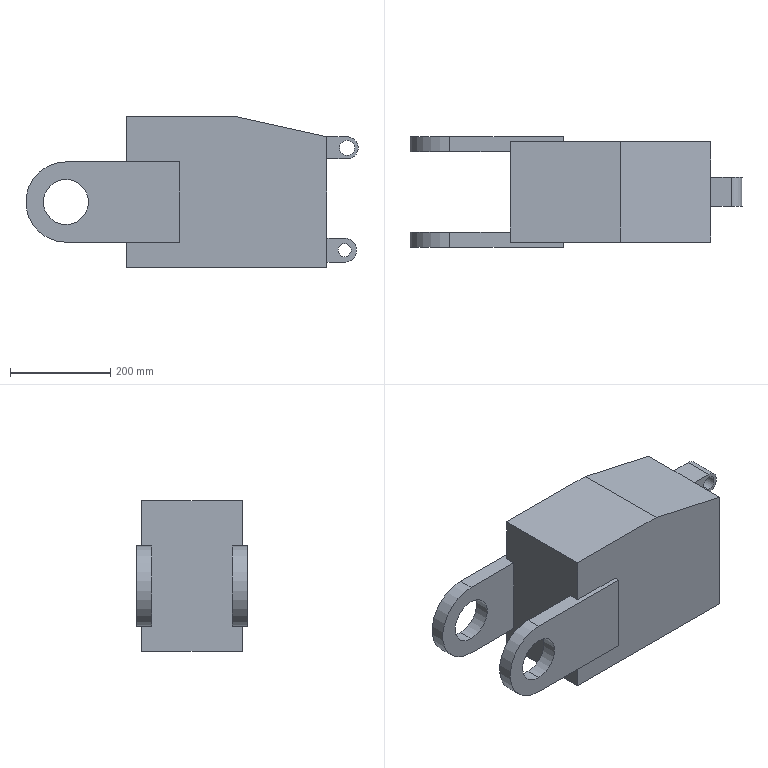Part | SolidWorks | features ICE 4, Extrusion 1, MirrorPattern 1 | 1 solid | 37 faces | box 662 x 220 x 300 mm | volume 25140960 mm3 | plane 25 | cylinder 12 | commonest cylinder face diameters 90 x4 26 x2 30 x2 160 x2 44 x1 48 x1
STEP:
#1=CARTESIAN_POINT('',(235.,90.,-129.));
#2=VERTEX_POINT('',#1);
#3=CARTESIAN_POINT('',(235.,90.,-103.));
#4=VERTEX_POINT('',#3);
#5=CARTESIAN_POINT('',(235.,90.,-116.));
#6=DIRECTION('',(0.,1.,0.));
#7=DIRECTION('',(0.,0.,1.));
#8=AXIS2_PLACEMENT_3D('',#5,#6,#7);
#9=CIRCLE('',#8,13.);
#10=EDGE_CURVE('',#2,#4,#9,.T.);
#11=ORIENTED_EDGE('',*,*,#10,.F.);
#12=CARTESIAN_POINT('',(235.,110.,-129.));
#13=VERTEX_POINT('',#12);
#14=CARTESIAN_POINT('',(235.,90.,-129.));
#15=DIRECTION('',(0.,1.,0.));
#16=VECTOR('',#15,1000.);
#17=LINE('',#14,#16);
#18=EDGE_CURVE('',#2,#13,#17,.T.);
#19=ORIENTED_EDGE('',*,*,#18,.T.);
#20=CARTESIAN_POINT('',(235.,110.,-103.));
#21=VERTEX_POINT('',#20);
#22=CARTESIAN_POINT('',(235.,110.,-116.));
#23=DIRECTION('',(0.,1.,0.));
#24=DIRECTION('',(0.,0.,1.));
#25=AXIS2_PLACEMENT_3D('',#22,#23,#24);
#26=CIRCLE('',#25,13.);
#27=EDGE_CURVE('',#13,#21,#26,.T.);
#28=ORIENTED_EDGE('',*,*,#27,.T.);
#29=CARTESIAN_POINT('',(235.,90.,-103.));
#30=DIRECTION('',(0.,1.,0.));
#31=VECTOR('',#30,1000.);
#32=LINE('',#29,#31);
#33=EDGE_CURVE('',#4,#21,#32,.T.);
#34=ORIENTED_EDGE('',*,*,#33,.F.);
#35=EDGE_LOOP('',(#11,#19,#28,#34));
#36=FACE_OUTER_BOUND('',#35,.T.);
#37=CARTESIAN_POINT('',(235.,90.,-116.));
#38=DIRECTION('',(0.,1.,0.));
#39=DIRECTION('',(0.,0.,1.));
#40=AXIS2_PLACEMENT_3D('',#37,#38,#39);
#41=CYLINDRICAL_SURFACE('',#40,13.);
#42=ADVANCED_FACE('',(#36),#41,.F.);
#43=CARTESIAN_POINT('',(-320.,-10.,-65.));
#44=VERTEX_POINT('',#43);
#45=CARTESIAN_POINT('',(-320.,-10.,25.));
#46=VERTEX_POINT('',#45);
#47=CARTESIAN_POINT('',(-320.,-10.,-20.));
#48=DIRECTION('',(0.,1.,0.));
#49=DIRECTION('',(0.,0.,1.));
#50=AXIS2_PLACEMENT_3D('',#47,#48,#49);
#51=CIRCLE('',#50,45.);
#52=EDGE_CURVE('',#44,#46,#51,.T.);
#53=ORIENTED_EDGE('',*,*,#52,.F.);
#54=CARTESIAN_POINT('',(-320.,20.,-65.));
#55=VERTEX_POINT('',#54);
#56=CARTESIAN_POINT('',(-320.,-10.,-65.));
#57=DIRECTION('',(0.,1.,0.));
#58=VECTOR('',#57,1000.);
#59=LINE('',#56,#58);
#60=EDGE_CURVE('',#44,#55,#59,.T.);
#61=ORIENTED_EDGE('',*,*,#60,.T.);
#62=CARTESIAN_POINT('',(-320.,20.,25.));
#63=VERTEX_POINT('',#62);
#64=CARTESIAN_POINT('',(-320.,20.,-20.));
#65=DIRECTION('',(0.,1.,0.));
#66=DIRECTION('',(0.,0.,1.));
#67=AXIS2_PLACEMENT_3D('',#64,#65,#66);
#68=CIRCLE('',#67,45.);
#69=EDGE_CURVE('',#55,#63,#68,.T.);
#70=ORIENTED_EDGE('',*,*,#69,.T.);
#71=CARTESIAN_POINT('',(-320.,-10.,25.));
#72=DIRECTION('',(0.,1.,0.));
#73=VECTOR('',#72,1000.);
#74=LINE('',#71,#73);
#75=EDGE_CURVE('',#46,#63,#74,.T.);
#76=ORIENTED_EDGE('',*,*,#75,.F.);
#77=EDGE_LOOP('',(#53,#61,#70,#76));
#78=FACE_OUTER_BOUND('',#77,.T.);
#79=CARTESIAN_POINT('',(-320.,-10.,-20.));
#80=DIRECTION('',(0.,1.,0.));
#81=DIRECTION('',(0.,0.,1.));
#82=AXIS2_PLACEMENT_3D('',#79,#80,#81);
#83=CYLINDRICAL_SURFACE('',#82,45.);
#84=ADVANCED_FACE('',(#78),#83,.F.);
#85=CARTESIAN_POINT('',(-320.,210.,-65.));
#86=VERTEX_POINT('',#85);
#87=CARTESIAN_POINT('',(-320.,210.,25.));
#88=VERTEX_POINT('',#87);
#89=CARTESIAN_POINT('',(-320.,210.,-20.));
#90=DIRECTION('',(0.,1.,0.));
#91=DIRECTION('',(0.,0.,1.));
#92=AXIS2_PLACEMENT_3D('',#89,#90,#91);
#93=CIRCLE('',#92,45.);
#94=EDGE_CURVE('',#86,#88,#93,.T.);
#95=ORIENTED_EDGE('',*,*,#94,.T.);
#96=CARTESIAN_POINT('',(-320.,180.,25.));
#97=VERTEX_POINT('',#96);
#98=CARTESIAN_POINT('',(-320.,210.,25.));
#99=DIRECTION('',(0.,-1.,0.));
#100=VECTOR('',#99,1000.);
#101=LINE('',#98,#100);
#102=EDGE_CURVE('',#88,#97,#101,.T.);
#103=ORIENTED_EDGE('',*,*,#102,.T.);
#104=CARTESIAN_POINT('',(-320.,180.,-65.));
#105=VERTEX_POINT('',#104);
#106=CARTESIAN_POINT('',(-320.,180.,-20.));
#107=DIRECTION('',(0.,1.,0.));
#108=DIRECTION('',(0.,0.,1.));
#109=AXIS2_PLACEMENT_3D('',#106,#107,#108);
#110=CIRCLE('',#109,45.);
#111=EDGE_CURVE('',#105,#97,#110,.T.);
#112=ORIENTED_EDGE('',*,*,#111,.F.);
#113=CARTESIAN_POINT('',(-320.,210.,-65.));
#114=DIRECTION('',(0.,-1.,0.));
#115=VECTOR('',#114,1000.);
#116=LINE('',#113,#115);
#117=EDGE_CURVE('',#86,#105,#116,.T.);
#118=ORIENTED_EDGE('',*,*,#117,.F.);
#119=EDGE_LOOP('',(#95,#103,#112,#118));
#120=FACE_OUTER_BOUND('',#119,.T.);
#121=CARTESIAN_POINT('',(-320.,210.,-20.));
#122=DIRECTION('',(0.,-1.,0.));
#123=DIRECTION('',(0.,0.,-1.));
#124=AXIS2_PLACEMENT_3D('',#121,#122,#123);
#125=CYLINDRICAL_SURFACE('',#124,45.);
#126=ADVANCED_FACE('',(#120),#125,.F.);
#127=CARTESIAN_POINT('',(240.,71.,73.));
#128=VERTEX_POINT('',#127);
#129=CARTESIAN_POINT('',(240.,71.,103.));
#130=VERTEX_POINT('',#129);
#131=CARTESIAN_POINT('',(240.,71.,88.));
#132=DIRECTION('',(0.,1.,0.));
#133=DIRECTION('',(0.,0.,1.));
#134=AXIS2_PLACEMENT_3D('',#131,#132,#133);
#135=CIRCLE('',#134,15.);
#136=EDGE_CURVE('',#128,#130,#135,.T.);
#137=ORIENTED_EDGE('',*,*,#136,.F.);
#138=CARTESIAN_POINT('',(240.,129.,73.));
#139=VERTEX_POINT('',#138);
#140=CARTESIAN_POINT('',(240.,71.,73.));
#141=DIRECTION('',(0.,1.,0.));
#142=VECTOR('',#141,1000.);
#143=LINE('',#140,#142);
#144=EDGE_CURVE('',#128,#139,#143,.T.);
#145=ORIENTED_EDGE('',*,*,#144,.T.);
#146=CARTESIAN_POINT('',(240.,129.,103.));
#147=VERTEX_POINT('',#146);
#148=CARTESIAN_POINT('',(240.,129.,88.));
#149=DIRECTION('',(0.,1.,0.));
#150=DIRECTION('',(0.,0.,1.));
#151=AXIS2_PLACEMENT_3D('',#148,#149,#150);
#152=CIRCLE('',#151,15.);
#153=EDGE_CURVE('',#139,#147,#152,.T.);
#154=ORIENTED_EDGE('',*,*,#153,.T.);
#155=CARTESIAN_POINT('',(240.,71.,103.));
#156=DIRECTION('',(0.,1.,0.));
#157=VECTOR('',#156,1000.);
#158=LINE('',#155,#157);
#159=EDGE_CURVE('',#130,#147,#158,.T.);
#160=ORIENTED_EDGE('',*,*,#159,.F.);
#161=EDGE_LOOP('',(#137,#145,#154,#160));
#162=FACE_OUTER_BOUND('',#161,.T.);
#163=CARTESIAN_POINT('',(240.,71.,88.));
#164=DIRECTION('',(0.,1.,0.));
#165=DIRECTION('',(0.,0.,1.));
#166=AXIS2_PLACEMENT_3D('',#163,#164,#165);
#167=CYLINDRICAL_SURFACE('',#166,15.);
#168=ADVANCED_FACE('',(#162),#167,.F.);
#169=CARTESIAN_POINT('',(200.,200.,110.));
#170=VERTEX_POINT('',#169);
#171=CARTESIAN_POINT('',(200.,200.,-150.));
#172=VERTEX_POINT('',#171);
#173=CARTESIAN_POINT('',(200.,200.,-150.));
#174=DIRECTION('',(0.,0.,-1.));
#175=VECTOR('',#174,1000.);
#176=LINE('',#173,#175);
#177=EDGE_CURVE('',#170,#172,#176,.T.);
#178=ORIENTED_EDGE('',*,*,#177,.F.);
#179=CARTESIAN_POINT('',(200.,129.,110.));
#180=VERTEX_POINT('',#179);
#181=CARTESIAN_POINT('',(200.,0.,110.));
#182=DIRECTION('',(0.,1.,0.));
#183=VECTOR('',#182,1000.);
#184=LINE('',#181,#183);
#185=EDGE_CURVE('',#180,#170,#184,.T.);
#186=ORIENTED_EDGE('',*,*,#185,.F.);
#187=CARTESIAN_POINT('',(200.,129.,66.));
#188=VERTEX_POINT('',#187);
#189=CARTESIAN_POINT('',(200.,129.,-150.));
#190=DIRECTION('',(0.,0.,-1.));
#191=VECTOR('',#190,1000.);
#192=LINE('',#189,#191);
#193=EDGE_CURVE('',#180,#188,#192,.T.);
#194=ORIENTED_EDGE('',*,*,#193,.T.);
#195=CARTESIAN_POINT('',(200.,71.,66.));
#196=VERTEX_POINT('',#195);
#197=CARTESIAN_POINT('',(200.,200.,66.));
#198=DIRECTION('',(0.,-1.,0.));
#199=VECTOR('',#198,1000.);
#200=LINE('',#197,#199);
#201=EDGE_CURVE('',#188,#196,#200,.T.);
#202=ORIENTED_EDGE('',*,*,#201,.T.);
#203=CARTESIAN_POINT('',(200.,71.,110.));
#204=VERTEX_POINT('',#203);
#205=CARTESIAN_POINT('',(200.,71.,-150.));
#206=DIRECTION('',(0.,0.,-1.));
#207=VECTOR('',#206,1000.);
#208=LINE('',#205,#207);
#209=EDGE_CURVE('',#204,#196,#208,.T.);
#210=ORIENTED_EDGE('',*,*,#209,.F.);
#211=CARTESIAN_POINT('',(200.,0.,110.));
#212=VERTEX_POINT('',#211);
#213=CARTESIAN_POINT('',(200.,0.,110.));
#214=DIRECTION('',(0.,1.,0.));
#215=VECTOR('',#214,1000.);
#216=LINE('',#213,#215);
#217=EDGE_CURVE('',#212,#204,#216,.T.);
#218=ORIENTED_EDGE('',*,*,#217,.F.);
#219=CARTESIAN_POINT('',(200.,0.,-150.));
#220=VERTEX_POINT('',#219);
#221=CARTESIAN_POINT('',(200.,0.,-150.));
#222=DIRECTION('',(0.,0.,-1.));
#223=VECTOR('',#222,1000.);
#224=LINE('',#221,#223);
#225=EDGE_CURVE('',#212,#220,#224,.T.);
#226=ORIENTED_EDGE('',*,*,#225,.T.);
#227=CARTESIAN_POINT('',(200.,200.,-150.));
#228=DIRECTION('',(0.,-1.,0.));
#229=VECTOR('',#228,1000.);
#230=LINE('',#227,#229);
#231=EDGE_CURVE('',#172,#220,#230,.T.);
#232=ORIENTED_EDGE('',*,*,#231,.F.);
#233=EDGE_LOOP('',(#178,#186,#194,#202,#210,#218,#226,#232));
#234=FACE_OUTER_BOUND('',#233,.T.);
#235=CARTESIAN_POINT('',(200.,90.,-92.));
#236=VERTEX_POINT('',#235);
#237=CARTESIAN_POINT('',(200.,90.,-140.));
#238=VERTEX_POINT('',#237);
#239=CARTESIAN_POINT('',(200.,90.,-150.));
#240=DIRECTION('',(0.,0.,-1.));
#241=VECTOR('',#240,1000.);
#242=LINE('',#239,#241);
#243=EDGE_CURVE('',#236,#238,#242,.T.);
#244=ORIENTED_EDGE('',*,*,#243,.F.);
#245=CARTESIAN_POINT('',(200.,110.,-92.));
#246=VERTEX_POINT('',#245);
#247=CARTESIAN_POINT('',(200.,200.,-92.));
#248=DIRECTION('',(0.,1.,0.));
#249=VECTOR('',#248,1000.);
#250=LINE('',#247,#249);
#251=EDGE_CURVE('',#236,#246,#250,.T.);
#252=ORIENTED_EDGE('',*,*,#251,.T.);
#253=CARTESIAN_POINT('',(200.,110.,-140.));
#254=VERTEX_POINT('',#253);
#255=CARTESIAN_POINT('',(200.,110.,-150.));
#256=DIRECTION('',(0.,0.,-1.));
#257=VECTOR('',#256,1000.);
#258=LINE('',#255,#257);
#259=EDGE_CURVE('',#246,#254,#258,.T.);
#260=ORIENTED_EDGE('',*,*,#259,.T.);
#261=CARTESIAN_POINT('',(200.,200.,-140.));
#262=DIRECTION('',(0.,-1.,0.));
#263=VECTOR('',#262,1000.);
#264=LINE('',#261,#263);
#265=EDGE_CURVE('',#254,#238,#264,.T.);
#266=ORIENTED_EDGE('',*,*,#265,.T.);
#267=EDGE_LOOP('',(#244,#252,#260,#266));
#268=FACE_BOUND('',#267,.T.);
#269=CARTESIAN_POINT('',(200.,200.,-150.));
#270=DIRECTION('',(-1.,0.,0.));
#271=DIRECTION('',(0.,0.,1.));
#272=AXIS2_PLACEMENT_3D('',#269,#270,#271);
#273=PLANE('',#272);
#274=ADVANCED_FACE('',(#234,#268),#273,.F.);
#275=CARTESIAN_POINT('',(-200.,20.,60.));
#276=VERTEX_POINT('',#275);
#277=CARTESIAN_POINT('',(-200.,20.,-100.));
#278=VERTEX_POINT('',#277);
#279=CARTESIAN_POINT('',(-200.,20.,-150.));
#280=DIRECTION('',(0.,0.,-1.));
#281=VECTOR('',#280,1000.);
#282=LINE('',#279,#281);
#283=EDGE_CURVE('',#276,#278,#282,.T.);
#284=ORIENTED_EDGE('',*,*,#283,.F.);
#285=CARTESIAN_POINT('',(-200.,0.,60.));
#286=VERTEX_POINT('',#285);
#287=CARTESIAN_POINT('',(-200.,200.,60.));
#288=DIRECTION('',(0.,-1.,0.));
#289=VECTOR('',#288,1000.);
#290=LINE('',#287,#289);
#291=EDGE_CURVE('',#276,#286,#290,.T.);
#292=ORIENTED_EDGE('',*,*,#291,.T.);
#293=CARTESIAN_POINT('',(-200.,0.,150.));
#294=VERTEX_POINT('',#293);
#295=CARTESIAN_POINT('',(-200.,0.,-150.));
#296=DIRECTION('',(0.,0.,1.));
#297=VECTOR('',#296,1000.);
#298=LINE('',#295,#297);
#299=EDGE_CURVE('',#286,#294,#298,.T.);
#300=ORIENTED_EDGE('',*,*,#299,.T.);
#301=CARTESIAN_POINT('',(-200.,200.,150.));
#302=VERTEX_POINT('',#301);
#303=CARTESIAN_POINT('',(-200.,200.,150.));
#304=DIRECTION('',(0.,-1.,0.));
#305=VECTOR('',#304,1000.);
#306=LINE('',#303,#305);
#307=EDGE_CURVE('',#302,#294,#306,.T.);
#308=ORIENTED_EDGE('',*,*,#307,.F.);
#309=CARTESIAN_POINT('',(-200.,200.,60.));
#310=VERTEX_POINT('',#309);
#311=CARTESIAN_POINT('',(-200.,200.,-150.));
#312=DIRECTION('',(0.,0.,1.));
#313=VECTOR('',#312,1000.);
#314=LINE('',#311,#313);
#315=EDGE_CURVE('',#310,#302,#314,.T.);
#316=ORIENTED_EDGE('',*,*,#315,.F.);
#317=CARTESIAN_POINT('',(-200.,180.,60.));
#318=VERTEX_POINT('',#317);
#319=CARTESIAN_POINT('',(-200.,200.,60.));
#320=DIRECTION('',(0.,1.,0.));
#321=VECTOR('',#320,1000.);
#322=LINE('',#319,#321);
#323=EDGE_CURVE('',#318,#310,#322,.T.);
#324=ORIENTED_EDGE('',*,*,#323,.F.);
#325=CARTESIAN_POINT('',(-200.,180.,-100.));
#326=VERTEX_POINT('',#325);
#327=CARTESIAN_POINT('',(-200.,180.,-150.));
#328=DIRECTION('',(0.,0.,1.));
#329=VECTOR('',#328,1000.);
#330=LINE('',#327,#329);
#331=EDGE_CURVE('',#326,#318,#330,.T.);
#332=ORIENTED_EDGE('',*,*,#331,.F.);
#333=CARTESIAN_POINT('',(-200.,200.,-100.));
#334=VERTEX_POINT('',#333);
#335=CARTESIAN_POINT('',(-200.,200.,-100.));
#336=DIRECTION('',(0.,-1.,0.));
#337=VECTOR('',#336,1000.);
#338=LINE('',#335,#337);
#339=EDGE_CURVE('',#334,#326,#338,.T.);
#340=ORIENTED_EDGE('',*,*,#339,.F.);
#341=CARTESIAN_POINT('',(-200.,200.,-150.));
#342=VERTEX_POINT('',#341);
#343=CARTESIAN_POINT('',(-200.,200.,-150.));
#344=DIRECTION('',(0.,0.,1.));
#345=VECTOR('',#344,1000.);
#346=LINE('',#343,#345);
#347=EDGE_CURVE('',#342,#334,#346,.T.);
#348=ORIENTED_EDGE('',*,*,#347,.F.);
#349=CARTESIAN_POINT('',(-200.,0.,-150.));
#350=VERTEX_POINT('',#349);
#351=CARTESIAN_POINT('',(-200.,200.,-150.));
#352=DIRECTION('',(0.,-1.,0.));
#353=VECTOR('',#352,1000.);
#354=LINE('',#351,#353);
#355=EDGE_CURVE('',#342,#350,#354,.T.);
#356=ORIENTED_EDGE('',*,*,#355,.T.);
#357=CARTESIAN_POINT('',(-200.,0.,-100.));
#358=VERTEX_POINT('',#357);
#359=CARTESIAN_POINT('',(-200.,0.,-150.));
#360=DIRECTION('',(0.,0.,1.));
#361=VECTOR('',#360,1000.);
#362=LINE('',#359,#361);
#363=EDGE_CURVE('',#350,#358,#362,.T.);
#364=ORIENTED_EDGE('',*,*,#363,.T.);
#365=CARTESIAN_POINT('',(-200.,200.,-100.));
#366=DIRECTION('',(0.,1.,0.));
#367=VECTOR('',#366,1000.);
#368=LINE('',#365,#367);
#369=EDGE_CURVE('',#358,#278,#368,.T.);
#370=ORIENTED_EDGE('',*,*,#369,.T.);
#371=EDGE_LOOP('',(#284,#292,#300,#308,#316,#324,#332,#340,#348,#356,#364,#370));
#372=FACE_OUTER_BOUND('',#371,.T.);
#373=CARTESIAN_POINT('',(-200.,200.,-150.));
#374=DIRECTION('',(1.,0.,0.));
#375=DIRECTION('',(0.,0.,-1.));
#376=AXIS2_PLACEMENT_3D('',#373,#374,#375);
#377=PLANE('',#376);
#378=ADVANCED_FACE('',(#372),#377,.F.);
#379=ORIENTED_EDGE('',*,*,#347,.T.);
#380=CARTESIAN_POINT('',(-94.279,200.,-100.));
#381=VERTEX_POINT('',#380);
#382=CARTESIAN_POINT('',(0.,200.,-100.));
#383=DIRECTION('',(1.,0.,0.));
#384=VECTOR('',#383,1000.);
#385=LINE('',#382,#384);
#386=EDGE_CURVE('',#334,#381,#385,.T.);
#387=ORIENTED_EDGE('',*,*,#386,.T.);
#388=CARTESIAN_POINT('',(-94.279,200.,60.));
#389=VERTEX_POINT('',#388);
#390=CARTESIAN_POINT('',(-94.279,200.,0.));
#391=DIRECTION('',(0.,0.,1.));
#392=VECTOR('',#391,1000.);
#393=LINE('',#390,#392);
#394=EDGE_CURVE('',#381,#389,#393,.T.);
#395=ORIENTED_EDGE('',*,*,#394,.T.);
#396=CARTESIAN_POINT('',(0.,200.,60.));
#397=DIRECTION('',(-1.,0.,0.));
#398=VECTOR('',#397,1000.);
#399=LINE('',#396,#398);
#400=EDGE_CURVE('',#389,#310,#399,.T.);
#401=ORIENTED_EDGE('',*,*,#400,.T.);
#402=ORIENTED_EDGE('',*,*,#315,.T.);
#403=CARTESIAN_POINT('',(20.729,200.,150.));
#404=VERTEX_POINT('',#403);
#405=CARTESIAN_POINT('',(-200.,200.,150.));
#406=DIRECTION('',(1.,0.,0.));
#407=VECTOR('',#406,1000.);
#408=LINE('',#405,#407);
#409=EDGE_CURVE('',#302,#404,#408,.T.);
#410=ORIENTED_EDGE('',*,*,#409,.T.);
#411=CARTESIAN_POINT('',(200.,200.,110.));
#412=DIRECTION('',(-0.976,0.,0.2178));
#413=VECTOR('',#412,1000.);
#414=LINE('',#411,#413);
#415=EDGE_CURVE('',#170,#404,#414,.T.);
#416=ORIENTED_EDGE('',*,*,#415,.F.);
#417=ORIENTED_EDGE('',*,*,#177,.T.);
#418=CARTESIAN_POINT('',(-200.,200.,-150.));
#419=DIRECTION('',(-1.,0.,0.));
#420=VECTOR('',#419,1000.);
#421=LINE('',#418,#420);
#422=EDGE_CURVE('',#172,#342,#421,.T.);
#423=ORIENTED_EDGE('',*,*,#422,.T.);
#424=EDGE_LOOP('',(#379,#387,#395,#401,#402,#410,#416,#417,#423));
#425=FACE_OUTER_BOUND('',#424,.T.);
#426=CARTESIAN_POINT('',(0.,200.,0.));
#427=DIRECTION('',(0.,1.,0.));
#428=DIRECTION('',(0.,0.,1.));
#429=AXIS2_PLACEMENT_3D('',#426,#427,#428);
#430=PLANE('',#429);
#431=ADVANCED_FACE('',(#425),#430,.T.);
#432=CARTESIAN_POINT('',(-200.,0.,-150.));
#433=DIRECTION('',(-1.,0.,0.));
#434=VECTOR('',#433,1000.);
#435=LINE('',#432,#434);
#436=EDGE_CURVE('',#220,#350,#435,.T.);
#437=ORIENTED_EDGE('',*,*,#436,.T.);
#438=ORIENTED_EDGE('',*,*,#355,.F.);
#439=ORIENTED_EDGE('',*,*,#422,.F.);
#440=ORIENTED_EDGE('',*,*,#231,.T.);
#441=EDGE_LOOP('',(#437,#438,#439,#440));
#442=FACE_OUTER_BOUND('',#441,.T.);
#443=CARTESIAN_POINT('',(-200.,200.,-150.));
#444=DIRECTION('',(0.,0.,1.));
#445=DIRECTION('',(1.,0.,0.));
#446=AXIS2_PLACEMENT_3D('',#443,#444,#445);
#447=PLANE('',#446);
#448=ADVANCED_FACE('',(#442),#447,.F.);
#449=CARTESIAN_POINT('',(20.729,0.,150.));
#450=VERTEX_POINT('',#449);
#451=CARTESIAN_POINT('',(-200.,0.,150.));
#452=DIRECTION('',(1.,0.,0.));
#453=VECTOR('',#452,1000.);
#454=LINE('',#451,#453);
#455=EDGE_CURVE('',#294,#450,#454,.T.);
#456=ORIENTED_EDGE('',*,*,#455,.T.);
#457=CARTESIAN_POINT('',(20.729,0.,150.));
#458=DIRECTION('',(0.,1.,0.));
#459=VECTOR('',#458,1000.);
#460=LINE('',#457,#459);
#461=EDGE_CURVE('',#450,#404,#460,.T.);
#462=ORIENTED_EDGE('',*,*,#461,.T.);
#463=ORIENTED_EDGE('',*,*,#409,.F.);
#464=ORIENTED_EDGE('',*,*,#307,.T.);
#465=EDGE_LOOP('',(#456,#462,#463,#464));
#466=FACE_OUTER_BOUND('',#465,.T.);
#467=CARTESIAN_POINT('',(-200.,200.,150.));
#468=DIRECTION('',(0.,0.,-1.));
#469=DIRECTION('',(-1.,0.,0.));
#470=AXIS2_PLACEMENT_3D('',#467,#468,#469);
#471=PLANE('',#470);
#472=ADVANCED_FACE('',(#466),#471,.F.);
#473=ORIENTED_EDGE('',*,*,#299,.F.);
#474=CARTESIAN_POINT('',(-94.279,0.,60.));
#475=VERTEX_POINT('',#474);
#476=CARTESIAN_POINT('',(0.,0.,60.));
#477=DIRECTION('',(1.,0.,0.));
#478=VECTOR('',#477,1000.);
#479=LINE('',#476,#478);
#480=EDGE_CURVE('',#286,#475,#479,.T.);
#481=ORIENTED_EDGE('',*,*,#480,.T.);
#482=CARTESIAN_POINT('',(-94.279,0.,-100.));
#483=VERTEX_POINT('',#482);
#484=CARTESIAN_POINT('',(-94.279,0.,0.));
#485=DIRECTION('',(0.,0.,-1.));
#486=VECTOR('',#485,1000.);
#487=LINE('',#484,#486);
#488=EDGE_CURVE('',#475,#483,#487,.T.);
#489=ORIENTED_EDGE('',*,*,#488,.T.);
#490=CARTESIAN_POINT('',(0.,0.,-100.));
#491=DIRECTION('',(-1.,0.,0.));
#492=VECTOR('',#491,1000.);
#493=LINE('',#490,#492);
#494=EDGE_CURVE('',#483,#358,#493,.T.);
#495=ORIENTED_EDGE('',*,*,#494,.T.);
#496=ORIENTED_EDGE('',*,*,#363,.F.);
#497=ORIENTED_EDGE('',*,*,#436,.F.);
#498=ORIENTED_EDGE('',*,*,#225,.F.);
#499=CARTESIAN_POINT('',(200.,0.,110.));
#500=DIRECTION('',(-0.976,0.,0.2178));
#501=VECTOR('',#500,1000.);
#502=LINE('',#499,#501);
#503=EDGE_CURVE('',#212,#450,#502,.T.);
#504=ORIENTED_EDGE('',*,*,#503,.T.);
#505=ORIENTED_EDGE('',*,*,#455,.F.);
#506=EDGE_LOOP('',(#473,#481,#489,#495,#496,#497,#498,#504,#505));
#507=FACE_OUTER_BOUND('',#506,.T.);
#508=CARTESIAN_POINT('',(0.,0.,0.));
#509=DIRECTION('',(0.,1.,0.));
#510=DIRECTION('',(0.,0.,1.));
#511=AXIS2_PLACEMENT_3D('',#508,#509,#510);
#512=PLANE('',#511);
#513=ADVANCED_FACE('',(#507),#512,.F.);
#514=CARTESIAN_POINT('',(200.,200.,110.));
#515=DIRECTION('',(0.,1.,0.));
#516=VECTOR('',#515,1000.);
#517=LINE('',#514,#516);
#518=EDGE_CURVE('',#204,#180,#517,.T.);
#519=ORIENTED_EDGE('',*,*,#518,.F.);
#520=CARTESIAN_POINT('',(240.,71.,110.));
#521=VERTEX_POINT('',#520);
#522=CARTESIAN_POINT('',(187.361,71.,110.));
#523=DIRECTION('',(1.,0.,0.));
#524=VECTOR('',#523,1000.);
#525=LINE('',#522,#524);
#526=EDGE_CURVE('',#204,#521,#525,.T.);
#527=ORIENTED_EDGE('',*,*,#526,.T.);
#528=CARTESIAN_POINT('',(240.,129.,110.));
#529=VERTEX_POINT('',#528);
#530=CARTESIAN_POINT('',(240.,71.,110.));
#531=DIRECTION('',(0.,1.,0.));
#532=VECTOR('',#531,1000.);
#533=LINE('',#530,#532);
#534=EDGE_CURVE('',#521,#529,#533,.T.);
#535=ORIENTED_EDGE('',*,*,#534,.T.);
#536=CARTESIAN_POINT('',(187.361,129.,110.));
#537=DIRECTION('',(1.,0.,0.));
#538=VECTOR('',#537,1000.);
#539=LINE('',#536,#538);
#540=EDGE_CURVE('',#180,#529,#539,.T.);
#541=ORIENTED_EDGE('',*,*,#540,.F.);
#542=EDGE_LOOP('',(#519,#527,#535,#541));
#543=FACE_OUTER_BOUND('',#542,.T.);
#544=CARTESIAN_POINT('',(187.361,71.,110.));
#545=DIRECTION('',(0.,0.,1.));
#546=DIRECTION('',(1.,0.,0.));
#547=AXIS2_PLACEMENT_3D('',#544,#545,#546);
#548=PLANE('',#547);
#549=ADVANCED_FACE('',(#543),#548,.T.);
#550=ORIENTED_EDGE('',*,*,#201,.F.);
#551=CARTESIAN_POINT('',(240.,129.,66.));
#552=VERTEX_POINT('',#551);
#553=CARTESIAN_POINT('',(187.361,129.,66.));
#554=DIRECTION('',(-1.,0.,0.));
#555=VECTOR('',#554,1000.);
#556=LINE('',#553,#555);
#557=EDGE_CURVE('',#552,#188,#556,.T.);
#558=ORIENTED_EDGE('',*,*,#557,.F.);
#559=CARTESIAN_POINT('',(240.,71.,66.));
#560=VERTEX_POINT('',#559);
#561=CARTESIAN_POINT('',(240.,71.,66.));
#562=DIRECTION('',(0.,1.,0.));
#563=VECTOR('',#562,1000.);
#564=LINE('',#561,#563);
#565=EDGE_CURVE('',#560,#552,#564,.T.);
#566=ORIENTED_EDGE('',*,*,#565,.F.);
#567=CARTESIAN_POINT('',(187.361,71.,66.));
#568=DIRECTION('',(-1.,0.,0.));
#569=VECTOR('',#568,1000.);
#570=LINE('',#567,#569);
#571=EDGE_CURVE('',#560,#196,#570,.T.);
#572=ORIENTED_EDGE('',*,*,#571,.T.);
#573=EDGE_LOOP('',(#550,#558,#566,#572));
#574=FACE_OUTER_BOUND('',#573,.T.);
#575=CARTESIAN_POINT('',(187.361,71.,66.));
#576=DIRECTION('',(0.,0.,-1.));
#577=DIRECTION('',(-1.,0.,0.));
#578=AXIS2_PLACEMENT_3D('',#575,#576,#577);
#579=PLANE('',#578);
#580=ADVANCED_FACE('',(#574),#579,.T.);
#581=CARTESIAN_POINT('',(240.,71.,88.));
#582=DIRECTION('',(0.,1.,0.));
#583=DIRECTION('',(0.,0.,1.));
#584=AXIS2_PLACEMENT_3D('',#581,#582,#583);
#585=CIRCLE('',#584,15.);
#586=EDGE_CURVE('',#130,#128,#585,.T.);
#587=ORIENTED_EDGE('',*,*,#586,.T.);
#588=ORIENTED_EDGE('',*,*,#136,.T.);
#589=EDGE_LOOP('',(#587,#588));
#590=FACE_BOUND('',#589,.T.);
#591=ORIENTED_EDGE('',*,*,#526,.F.);
#592=ORIENTED_EDGE('',*,*,#209,.T.);
#593=ORIENTED_EDGE('',*,*,#571,.F.);
#594=CARTESIAN_POINT('',(240.,71.,88.));
#595=DIRECTION('',(0.,1.,0.));
#596=DIRECTION('',(0.,0.,1.));
#597=AXIS2_PLACEMENT_3D('',#594,#595,#596);
#598=CIRCLE('',#597,22.);
#599=EDGE_CURVE('',#521,#560,#598,.T.);
#600=ORIENTED_EDGE('',*,*,#599,.F.);
#601=EDGE_LOOP('',(#591,#592,#593,#600));
#602=FACE_OUTER_BOUND('',#601,.T.);
#603=CARTESIAN_POINT('',(240.,71.,88.));
#604=DIRECTION('',(0.,1.,0.));
#605=DIRECTION('',(0.,0.,1.));
#606=AXIS2_PLACEMENT_3D('',#603,#604,#605);
#607=PLANE('',#606);
#608=ADVANCED_FACE('',(#590,#602),#607,.F.);
#609=CARTESIAN_POINT('',(240.,129.,88.));
#610=DIRECTION('',(0.,1.,0.));
#611=DIRECTION('',(0.,0.,1.));
#612=AXIS2_PLACEMENT_3D('',#609,#610,#611);
#613=CIRCLE('',#612,15.);
#614=EDGE_CURVE('',#147,#139,#613,.T.);
#615=ORIENTED_EDGE('',*,*,#614,.F.);
#616=ORIENTED_EDGE('',*,*,#153,.F.);
#617=EDGE_LOOP('',(#615,#616));
#618=FACE_BOUND('',#617,.T.);
#619=ORIENTED_EDGE('',*,*,#193,.F.);
#620=ORIENTED_EDGE('',*,*,#540,.T.);
#621=CARTESIAN_POINT('',(240.,129.,88.));
#622=DIRECTION('',(0.,1.,0.));
#623=DIRECTION('',(0.,0.,1.));
#624=AXIS2_PLACEMENT_3D('',#621,#622,#623);
#625=CIRCLE('',#624,22.);
#626=EDGE_CURVE('',#529,#552,#625,.T.);
#627=ORIENTED_EDGE('',*,*,#626,.T.);
#628=ORIENTED_EDGE('',*,*,#557,.T.);
#629=EDGE_LOOP('',(#619,#620,#627,#628));
#630=FACE_OUTER_BOUND('',#629,.T.);
#631=CARTESIAN_POINT('',(240.,129.,88.));
#632=DIRECTION('',(0.,1.,0.));
#633=DIRECTION('',(0.,0.,1.));
#634=AXIS2_PLACEMENT_3D('',#631,#632,#633);
#635=PLANE('',#634);
#636=ADVANCED_FACE('',(#618,#630),#635,.T.);
#637=ORIENTED_EDGE('',*,*,#565,.T.);
#638=ORIENTED_EDGE('',*,*,#626,.F.);
#639=ORIENTED_EDGE('',*,*,#534,.F.);
#640=ORIENTED_EDGE('',*,*,#599,.T.);
#641=EDGE_LOOP('',(#637,#638,#639,#640));
#642=FACE_OUTER_BOUND('',#641,.T.);
#643=CARTESIAN_POINT('',(240.,71.,88.));
#644=DIRECTION('',(0.,1.,0.));
#645=DIRECTION('',(0.,0.,1.));
#646=AXIS2_PLACEMENT_3D('',#643,#644,#645);
#647=CYLINDRICAL_SURFACE('',#646,22.);
#648=ADVANCED_FACE('',(#642),#647,.T.);
#649=ORIENTED_EDGE('',*,*,#144,.F.);
#650=ORIENTED_EDGE('',*,*,#586,.F.);
#651=ORIENTED_EDGE('',*,*,#159,.T.);
#652=ORIENTED_EDGE('',*,*,#614,.T.);
#653=EDGE_LOOP('',(#649,#650,#651,#652));
#654=FACE_OUTER_BOUND('',#653,.T.);
#655=CARTESIAN_POINT('',(240.,71.,88.));
#656=DIRECTION('',(0.,1.,0.));
#657=DIRECTION('',(0.,0.,1.));
#658=AXIS2_PLACEMENT_3D('',#655,#656,#657);
#659=CYLINDRICAL_SURFACE('',#658,15.);
#660=ADVANCED_FACE('',(#654),#659,.F.);
#661=ORIENTED_EDGE('',*,*,#415,.T.);
#662=ORIENTED_EDGE('',*,*,#461,.F.);
#663=ORIENTED_EDGE('',*,*,#503,.F.);
#664=ORIENTED_EDGE('',*,*,#217,.T.);
#665=ORIENTED_EDGE('',*,*,#518,.T.);
#666=ORIENTED_EDGE('',*,*,#185,.T.);
#667=EDGE_LOOP('',(#661,#662,#663,#664,#665,#666));
#668=FACE_OUTER_BOUND('',#667,.T.);
#669=CARTESIAN_POINT('',(200.,0.,110.));
#670=DIRECTION('',(-0.2178,0.,-0.976));
#671=DIRECTION('',(-0.976,0.,0.2178));
#672=AXIS2_PLACEMENT_3D('',#669,#670,#671);
#673=PLANE('',#672);
#674=ADVANCED_FACE('',(#668),#673,.F.);
#675=ORIENTED_EDGE('',*,*,#111,.T.);
#676=CARTESIAN_POINT('',(-320.,180.,-20.));
#677=DIRECTION('',(0.,1.,0.));
#678=DIRECTION('',(0.,0.,1.));
#679=AXIS2_PLACEMENT_3D('',#676,#677,#678);
#680=CIRCLE('',#679,45.);
#681=EDGE_CURVE('',#97,#105,#680,.T.);
#682=ORIENTED_EDGE('',*,*,#681,.T.);
#683=EDGE_LOOP('',(#675,#682));
#684=FACE_BOUND('',#683,.T.);
#685=CARTESIAN_POINT('',(-320.,180.,-100.));
#686=VERTEX_POINT('',#685);
#687=CARTESIAN_POINT('',(-94.279,180.,-100.));
#688=DIRECTION('',(-1.,0.,0.));
#689=VECTOR('',#688,1000.);
#690=LINE('',#687,#689);
#691=EDGE_CURVE('',#326,#686,#690,.T.);
#692=ORIENTED_EDGE('',*,*,#691,.F.);
#693=ORIENTED_EDGE('',*,*,#331,.T.);
#694=CARTESIAN_POINT('',(-320.,180.,60.));
#695=VERTEX_POINT('',#694);
#696=CARTESIAN_POINT('',(-94.279,180.,60.));
#697=DIRECTION('',(1.,0.,0.));
#698=VECTOR('',#697,1000.);
#699=LINE('',#696,#698);
#700=EDGE_CURVE('',#695,#318,#699,.T.);
#701=ORIENTED_EDGE('',*,*,#700,.F.);
#702=CARTESIAN_POINT('',(-320.,180.,-20.));
#703=DIRECTION('',(0.,1.,0.));
#704=DIRECTION('',(0.,0.,1.));
#705=AXIS2_PLACEMENT_3D('',#702,#703,#704);
#706=CIRCLE('',#705,80.);
#707=EDGE_CURVE('',#686,#695,#706,.T.);
#708=ORIENTED_EDGE('',*,*,#707,.F.);
#709=EDGE_LOOP('',(#692,#693,#701,#708));
#710=FACE_OUTER_BOUND('',#709,.T.);
#711=CARTESIAN_POINT('',(-320.,180.,-20.));
#712=DIRECTION('',(0.,1.,0.));
#713=DIRECTION('',(0.,0.,1.));
#714=AXIS2_PLACEMENT_3D('',#711,#712,#713);
#715=PLANE('',#714);
#716=ADVANCED_FACE('',(#684,#710),#715,.F.);
#717=ORIENTED_EDGE('',*,*,#386,.F.);
#718=ORIENTED_EDGE('',*,*,#339,.T.);
#719=ORIENTED_EDGE('',*,*,#691,.T.);
#720=CARTESIAN_POINT('',(-320.,210.,-100.));
#721=VERTEX_POINT('',#720);
#722=CARTESIAN_POINT('',(-320.,210.,-100.));
#723=DIRECTION('',(0.,-1.,0.));
#724=VECTOR('',#723,1000.);
#725=LINE('',#722,#724);
#726=EDGE_CURVE('',#721,#686,#725,.T.);
#727=ORIENTED_EDGE('',*,*,#726,.F.);
#728=CARTESIAN_POINT('',(-94.279,210.,-100.));
#729=VERTEX_POINT('',#728);
#730=CARTESIAN_POINT('',(-94.279,210.,-100.));
#731=DIRECTION('',(-1.,0.,0.));
#732=VECTOR('',#731,1000.);
#733=LINE('',#730,#732);
#734=EDGE_CURVE('',#729,#721,#733,.T.);
#735=ORIENTED_EDGE('',*,*,#734,.F.);
#736=CARTESIAN_POINT('',(-94.279,210.,-100.));
#737=DIRECTION('',(0.,-1.,0.));
#738=VECTOR('',#737,1000.);
#739=LINE('',#736,#738);
#740=EDGE_CURVE('',#729,#381,#739,.T.);
#741=ORIENTED_EDGE('',*,*,#740,.T.);
#742=EDGE_LOOP('',(#717,#718,#719,#727,#735,#741));
#743=FACE_OUTER_BOUND('',#742,.T.);
#744=CARTESIAN_POINT('',(-94.279,210.,-100.));
#745=DIRECTION('',(0.,0.,1.));
#746=DIRECTION('',(1.,0.,0.));
#747=AXIS2_PLACEMENT_3D('',#744,#745,#746);
#748=PLANE('',#747);
#749=ADVANCED_FACE('',(#743),#748,.F.);
#750=ORIENTED_EDGE('',*,*,#700,.T.);
#751=ORIENTED_EDGE('',*,*,#323,.T.);
#752=ORIENTED_EDGE('',*,*,#400,.F.);
#753=CARTESIAN_POINT('',(-94.279,210.,60.));
#754=VERTEX_POINT('',#753);
#755=CARTESIAN_POINT('',(-94.279,210.,60.));
#756=DIRECTION('',(0.,-1.,0.));
#757=VECTOR('',#756,1000.);
#758=LINE('',#755,#757);
#759=EDGE_CURVE('',#754,#389,#758,.T.);
#760=ORIENTED_EDGE('',*,*,#759,.F.);
#761=CARTESIAN_POINT('',(-320.,210.,60.));
#762=VERTEX_POINT('',#761);
#763=CARTESIAN_POINT('',(-94.279,210.,60.));
#764=DIRECTION('',(1.,0.,0.));
#765=VECTOR('',#764,1000.);
#766=LINE('',#763,#765);
#767=EDGE_CURVE('',#762,#754,#766,.T.);
#768=ORIENTED_EDGE('',*,*,#767,.F.);
#769=CARTESIAN_POINT('',(-320.,210.,60.));
#770=DIRECTION('',(0.,-1.,0.));
#771=VECTOR('',#770,1000.);
#772=LINE('',#769,#771);
#773=EDGE_CURVE('',#762,#695,#772,.T.);
#774=ORIENTED_EDGE('',*,*,#773,.T.);
#775=EDGE_LOOP('',(#750,#751,#752,#760,#768,#774));
#776=FACE_OUTER_BOUND('',#775,.T.);
#777=CARTESIAN_POINT('',(-94.279,210.,60.));
#778=DIRECTION('',(0.,0.,-1.));
#779=DIRECTION('',(-1.,0.,0.));
#780=AXIS2_PLACEMENT_3D('',#777,#778,#779);
#781=PLANE('',#780);
#782=ADVANCED_FACE('',(#776),#781,.F.);
#783=CARTESIAN_POINT('',(-94.279,210.,-100.));
#784=DIRECTION('',(0.,0.,-1.));
#785=VECTOR('',#784,1000.);
#786=LINE('',#783,#785);
#787=EDGE_CURVE('',#754,#729,#786,.T.);
#788=ORIENTED_EDGE('',*,*,#787,.T.);
#789=ORIENTED_EDGE('',*,*,#734,.T.);
#790=CARTESIAN_POINT('',(-320.,210.,-20.));
#791=DIRECTION('',(0.,1.,0.));
#792=DIRECTION('',(0.,0.,1.));
#793=AXIS2_PLACEMENT_3D('',#790,#791,#792);
#794=CIRCLE('',#793,80.);
#795=EDGE_CURVE('',#721,#762,#794,.T.);
#796=ORIENTED_EDGE('',*,*,#795,.T.);
#797=ORIENTED_EDGE('',*,*,#767,.T.);
#798=EDGE_LOOP('',(#788,#789,#796,#797));
#799=FACE_OUTER_BOUND('',#798,.T.);
#800=ORIENTED_EDGE('',*,*,#94,.F.);
#801=CARTESIAN_POINT('',(-320.,210.,-20.));
#802=DIRECTION('',(0.,1.,0.));
#803=DIRECTION('',(0.,0.,1.));
#804=AXIS2_PLACEMENT_3D('',#801,#802,#803);
#805=CIRCLE('',#804,45.);
#806=EDGE_CURVE('',#88,#86,#805,.T.);
#807=ORIENTED_EDGE('',*,*,#806,.F.);
#808=EDGE_LOOP('',(#800,#807));
#809=FACE_BOUND('',#808,.T.);
#810=CARTESIAN_POINT('',(-320.,210.,-20.));
#811=DIRECTION('',(0.,1.,0.));
#812=DIRECTION('',(0.,0.,1.));
#813=AXIS2_PLACEMENT_3D('',#810,#811,#812);
#814=PLANE('',#813);
#815=ADVANCED_FACE('',(#799,#809),#814,.T.);
#816=ORIENTED_EDGE('',*,*,#394,.F.);
#817=ORIENTED_EDGE('',*,*,#740,.F.);
#818=ORIENTED_EDGE('',*,*,#787,.F.);
#819=ORIENTED_EDGE('',*,*,#759,.T.);
#820=EDGE_LOOP('',(#816,#817,#818,#819));
#821=FACE_OUTER_BOUND('',#820,.T.);
#822=CARTESIAN_POINT('',(-94.279,210.,-100.));
#823=DIRECTION('',(-1.,0.,0.));
#824=DIRECTION('',(0.,0.,1.));
#825=AXIS2_PLACEMENT_3D('',#822,#823,#824);
#826=PLANE('',#825);
#827=ADVANCED_FACE('',(#821),#826,.F.);
#828=ORIENTED_EDGE('',*,*,#726,.T.);
#829=ORIENTED_EDGE('',*,*,#707,.T.);
#830=ORIENTED_EDGE('',*,*,#773,.F.);
#831=ORIENTED_EDGE('',*,*,#795,.F.);
#832=EDGE_LOOP('',(#828,#829,#830,#831));
#833=FACE_OUTER_BOUND('',#832,.T.);
#834=CARTESIAN_POINT('',(-320.,210.,-20.));
#835=DIRECTION('',(0.,-1.,0.));
#836=DIRECTION('',(0.,0.,-1.));
#837=AXIS2_PLACEMENT_3D('',#834,#835,#836);
#838=CYLINDRICAL_SURFACE('',#837,80.);
#839=ADVANCED_FACE('',(#833),#838,.T.);
#840=ORIENTED_EDGE('',*,*,#102,.F.);
#841=ORIENTED_EDGE('',*,*,#806,.T.);
#842=ORIENTED_EDGE('',*,*,#117,.T.);
#843=ORIENTED_EDGE('',*,*,#681,.F.);
#844=EDGE_LOOP('',(#840,#841,#842,#843));
#845=FACE_OUTER_BOUND('',#844,.T.);
#846=CARTESIAN_POINT('',(-320.,210.,-20.));
#847=DIRECTION('',(0.,-1.,0.));
#848=DIRECTION('',(0.,0.,-1.));
#849=AXIS2_PLACEMENT_3D('',#846,#847,#848);
#850=CYLINDRICAL_SURFACE('',#849,45.);
#851=ADVANCED_FACE('',(#845),#850,.F.);
#852=CARTESIAN_POINT('',(-320.,20.,-20.));
#853=DIRECTION('',(0.,1.,0.));
#854=DIRECTION('',(0.,0.,1.));
#855=AXIS2_PLACEMENT_3D('',#852,#853,#854);
#856=CIRCLE('',#855,45.);
#857=EDGE_CURVE('',#63,#55,#856,.T.);
#858=ORIENTED_EDGE('',*,*,#857,.F.);
#859=ORIENTED_EDGE('',*,*,#69,.F.);
#860=EDGE_LOOP('',(#858,#859));
#861=FACE_BOUND('',#860,.T.);
#862=CARTESIAN_POINT('',(-320.,20.,60.));
#863=VERTEX_POINT('',#862);
#864=CARTESIAN_POINT('',(-94.279,20.,60.));
#865=DIRECTION('',(1.,0.,0.));
#866=VECTOR('',#865,1000.);
#867=LINE('',#864,#866);
#868=EDGE_CURVE('',#863,#276,#867,.T.);
#869=ORIENTED_EDGE('',*,*,#868,.T.);
#870=ORIENTED_EDGE('',*,*,#283,.T.);
#871=CARTESIAN_POINT('',(-320.,20.,-100.));
#872=VERTEX_POINT('',#871);
#873=CARTESIAN_POINT('',(-94.279,20.,-100.));
#874=DIRECTION('',(-1.,0.,0.));
#875=VECTOR('',#874,1000.);
#876=LINE('',#873,#875);
#877=EDGE_CURVE('',#278,#872,#876,.T.);
#878=ORIENTED_EDGE('',*,*,#877,.T.);
#879=CARTESIAN_POINT('',(-320.,20.,-20.));
#880=DIRECTION('',(0.,1.,0.));
#881=DIRECTION('',(0.,0.,1.));
#882=AXIS2_PLACEMENT_3D('',#879,#880,#881);
#883=CIRCLE('',#882,80.);
#884=EDGE_CURVE('',#872,#863,#883,.T.);
#885=ORIENTED_EDGE('',*,*,#884,.T.);
#886=EDGE_LOOP('',(#869,#870,#878,#885));
#887=FACE_OUTER_BOUND('',#886,.T.);
#888=CARTESIAN_POINT('',(-320.,20.,-20.));
#889=DIRECTION('',(0.,-1.,0.));
#890=DIRECTION('',(0.,0.,1.));
#891=AXIS2_PLACEMENT_3D('',#888,#889,#890);
#892=PLANE('',#891);
#893=ADVANCED_FACE('',(#861,#887),#892,.F.);
#894=ORIENTED_EDGE('',*,*,#488,.F.);
#895=CARTESIAN_POINT('',(-94.279,-10.,60.));
#896=VERTEX_POINT('',#895);
#897=CARTESIAN_POINT('',(-94.279,-10.,60.));
#898=DIRECTION('',(0.,1.,0.));
#899=VECTOR('',#898,1000.);
#900=LINE('',#897,#899);
#901=EDGE_CURVE('',#896,#475,#900,.T.);
#902=ORIENTED_EDGE('',*,*,#901,.F.);
#903=CARTESIAN_POINT('',(-94.279,-10.,-100.));
#904=VERTEX_POINT('',#903);
#905=CARTESIAN_POINT('',(-94.279,-10.,-100.));
#906=DIRECTION('',(0.,0.,-1.));
#907=VECTOR('',#906,1000.);
#908=LINE('',#905,#907);
#909=EDGE_CURVE('',#896,#904,#908,.T.);
#910=ORIENTED_EDGE('',*,*,#909,.T.);
#911=CARTESIAN_POINT('',(-94.279,-10.,-100.));
#912=DIRECTION('',(0.,1.,0.));
#913=VECTOR('',#912,1000.);
#914=LINE('',#911,#913);
#915=EDGE_CURVE('',#904,#483,#914,.T.);
#916=ORIENTED_EDGE('',*,*,#915,.T.);
#917=EDGE_LOOP('',(#894,#902,#910,#916));
#918=FACE_OUTER_BOUND('',#917,.T.);
#919=CARTESIAN_POINT('',(-94.279,-10.,-100.));
#920=DIRECTION('',(1.,0.,0.));
#921=DIRECTION('',(0.,0.,-1.));
#922=AXIS2_PLACEMENT_3D('',#919,#920,#921);
#923=PLANE('',#922);
#924=ADVANCED_FACE('',(#918),#923,.T.);
#925=ORIENTED_EDGE('',*,*,#291,.F.);
#926=ORIENTED_EDGE('',*,*,#868,.F.);
#927=CARTESIAN_POINT('',(-320.,-10.,60.));
#928=VERTEX_POINT('',#927);
#929=CARTESIAN_POINT('',(-320.,-10.,60.));
#930=DIRECTION('',(0.,1.,0.));
#931=VECTOR('',#930,1000.);
#932=LINE('',#929,#931);
#933=EDGE_CURVE('',#928,#863,#932,.T.);
#934=ORIENTED_EDGE('',*,*,#933,.F.);
#935=CARTESIAN_POINT('',(-94.279,-10.,60.));
#936=DIRECTION('',(1.,0.,0.));
#937=VECTOR('',#936,1000.);
#938=LINE('',#935,#937);
#939=EDGE_CURVE('',#928,#896,#938,.T.);
#940=ORIENTED_EDGE('',*,*,#939,.T.);
#941=ORIENTED_EDGE('',*,*,#901,.T.);
#942=ORIENTED_EDGE('',*,*,#480,.F.);
#943=EDGE_LOOP('',(#925,#926,#934,#940,#941,#942));
#944=FACE_OUTER_BOUND('',#943,.T.);
#945=CARTESIAN_POINT('',(-94.279,-10.,60.));
#946=DIRECTION('',(0.,0.,1.));
#947=DIRECTION('',(1.,0.,0.));
#948=AXIS2_PLACEMENT_3D('',#945,#946,#947);
#949=PLANE('',#948);
#950=ADVANCED_FACE('',(#944),#949,.T.);
#951=ORIENTED_EDGE('',*,*,#369,.F.);
#952=ORIENTED_EDGE('',*,*,#494,.F.);
#953=ORIENTED_EDGE('',*,*,#915,.F.);
#954=CARTESIAN_POINT('',(-320.,-10.,-100.));
#955=VERTEX_POINT('',#954);
#956=CARTESIAN_POINT('',(-94.279,-10.,-100.));
#957=DIRECTION('',(-1.,0.,0.));
#958=VECTOR('',#957,1000.);
#959=LINE('',#956,#958);
#960=EDGE_CURVE('',#904,#955,#959,.T.);
#961=ORIENTED_EDGE('',*,*,#960,.T.);
#962=CARTESIAN_POINT('',(-320.,-10.,-100.));
#963=DIRECTION('',(0.,1.,0.));
#964=VECTOR('',#963,1000.);
#965=LINE('',#962,#964);
#966=EDGE_CURVE('',#955,#872,#965,.T.);
#967=ORIENTED_EDGE('',*,*,#966,.T.);
#968=ORIENTED_EDGE('',*,*,#877,.F.);
#969=EDGE_LOOP('',(#951,#952,#953,#961,#967,#968));
#970=FACE_OUTER_BOUND('',#969,.T.);
#971=CARTESIAN_POINT('',(-94.279,-10.,-100.));
#972=DIRECTION('',(0.,0.,-1.));
#973=DIRECTION('',(-1.,0.,0.));
#974=AXIS2_PLACEMENT_3D('',#971,#972,#973);
#975=PLANE('',#974);
#976=ADVANCED_FACE('',(#970),#975,.T.);
#977=ORIENTED_EDGE('',*,*,#933,.T.);
#978=ORIENTED_EDGE('',*,*,#884,.F.);
#979=ORIENTED_EDGE('',*,*,#966,.F.);
#980=CARTESIAN_POINT('',(-320.,-10.,-20.));
#981=DIRECTION('',(0.,1.,0.));
#982=DIRECTION('',(0.,0.,1.));
#983=AXIS2_PLACEMENT_3D('',#980,#981,#982);
#984=CIRCLE('',#983,80.);
#985=EDGE_CURVE('',#955,#928,#984,.T.);
#986=ORIENTED_EDGE('',*,*,#985,.T.);
#987=EDGE_LOOP('',(#977,#978,#979,#986));
#988=FACE_OUTER_BOUND('',#987,.T.);
#989=CARTESIAN_POINT('',(-320.,-10.,-20.));
#990=DIRECTION('',(0.,1.,0.));
#991=DIRECTION('',(0.,0.,1.));
#992=AXIS2_PLACEMENT_3D('',#989,#990,#991);
#993=CYLINDRICAL_SURFACE('',#992,80.);
#994=ADVANCED_FACE('',(#988),#993,.T.);
#995=CARTESIAN_POINT('',(-320.,-10.,-20.));
#996=DIRECTION('',(0.,1.,0.));
#997=DIRECTION('',(0.,0.,1.));
#998=AXIS2_PLACEMENT_3D('',#995,#996,#997);
#999=CIRCLE('',#998,45.);
#1000=EDGE_CURVE('',#46,#44,#999,.T.);
#1001=ORIENTED_EDGE('',*,*,#1000,.T.);
#1002=ORIENTED_EDGE('',*,*,#52,.T.);
#1003=EDGE_LOOP('',(#1001,#1002));
#1004=FACE_BOUND('',#1003,.T.);
#1005=ORIENTED_EDGE('',*,*,#909,.F.);
#1006=ORIENTED_EDGE('',*,*,#939,.F.);
#1007=ORIENTED_EDGE('',*,*,#985,.F.);
#1008=ORIENTED_EDGE('',*,*,#960,.F.);
#1009=EDGE_LOOP('',(#1005,#1006,#1007,#1008));
#1010=FACE_OUTER_BOUND('',#1009,.T.);
#1011=CARTESIAN_POINT('',(-320.,-10.,-20.));
#1012=DIRECTION('',(0.,-1.,0.));
#1013=DIRECTION('',(0.,0.,1.));
#1014=AXIS2_PLACEMENT_3D('',#1011,#1012,#1013);
#1015=PLANE('',#1014);
#1016=ADVANCED_FACE('',(#1004,#1010),#1015,.T.);
#1017=ORIENTED_EDGE('',*,*,#60,.F.);
#1018=ORIENTED_EDGE('',*,*,#1000,.F.);
#1019=ORIENTED_EDGE('',*,*,#75,.T.);
#1020=ORIENTED_EDGE('',*,*,#857,.T.);
#1021=EDGE_LOOP('',(#1017,#1018,#1019,#1020));
#1022=FACE_OUTER_BOUND('',#1021,.T.);
#1023=CARTESIAN_POINT('',(-320.,-10.,-20.));
#1024=DIRECTION('',(0.,1.,0.));
#1025=DIRECTION('',(0.,0.,1.));
#1026=AXIS2_PLACEMENT_3D('',#1023,#1024,#1025);
#1027=CYLINDRICAL_SURFACE('',#1026,45.);
#1028=ADVANCED_FACE('',(#1022),#1027,.F.);
#1029=ORIENTED_EDGE('',*,*,#251,.F.);
#1030=CARTESIAN_POINT('',(235.,90.,-92.));
#1031=VERTEX_POINT('',#1030);
#1032=CARTESIAN_POINT('',(184.248,90.,-92.));
#1033=DIRECTION('',(1.,0.,0.));
#1034=VECTOR('',#1033,1000.);
#1035=LINE('',#1032,#1034);
#1036=EDGE_CURVE('',#236,#1031,#1035,.T.);
#1037=ORIENTED_EDGE('',*,*,#1036,.T.);
#1038=CARTESIAN_POINT('',(235.,110.,-92.));
#1039=VERTEX_POINT('',#1038);
#1040=CARTESIAN_POINT('',(235.,90.,-92.));
#1041=DIRECTION('',(0.,1.,0.));
#1042=VECTOR('',#1041,1000.);
#1043=LINE('',#1040,#1042);
#1044=EDGE_CURVE('',#1031,#1039,#1043,.T.);
#1045=ORIENTED_EDGE('',*,*,#1044,.T.);
#1046=CARTESIAN_POINT('',(184.248,110.,-92.));
#1047=DIRECTION('',(1.,0.,0.));
#1048=VECTOR('',#1047,1000.);
#1049=LINE('',#1046,#1048);
#1050=EDGE_CURVE('',#246,#1039,#1049,.T.);
#1051=ORIENTED_EDGE('',*,*,#1050,.F.);
#1052=EDGE_LOOP('',(#1029,#1037,#1045,#1051));
#1053=FACE_OUTER_BOUND('',#1052,.T.);
#1054=CARTESIAN_POINT('',(184.248,90.,-92.));
#1055=DIRECTION('',(0.,0.,1.));
#1056=DIRECTION('',(1.,0.,0.));
#1057=AXIS2_PLACEMENT_3D('',#1054,#1055,#1056);
#1058=PLANE('',#1057);
#1059=ADVANCED_FACE('',(#1053),#1058,.T.);
#1060=ORIENTED_EDGE('',*,*,#265,.F.);
#1061=CARTESIAN_POINT('',(235.,110.,-140.));
#1062=VERTEX_POINT('',#1061);
#1063=CARTESIAN_POINT('',(184.248,110.,-140.));
#1064=DIRECTION('',(-1.,0.,0.));
#1065=VECTOR('',#1064,1000.);
#1066=LINE('',#1063,#1065);
#1067=EDGE_CURVE('',#1062,#254,#1066,.T.);
#1068=ORIENTED_EDGE('',*,*,#1067,.F.);
#1069=CARTESIAN_POINT('',(235.,90.,-140.));
#1070=VERTEX_POINT('',#1069);
#1071=CARTESIAN_POINT('',(235.,90.,-140.));
#1072=DIRECTION('',(0.,1.,0.));
#1073=VECTOR('',#1072,1000.);
#1074=LINE('',#1071,#1073);
#1075=EDGE_CURVE('',#1070,#1062,#1074,.T.);
#1076=ORIENTED_EDGE('',*,*,#1075,.F.);
#1077=CARTESIAN_POINT('',(184.248,90.,-140.));
#1078=DIRECTION('',(-1.,0.,0.));
#1079=VECTOR('',#1078,1000.);
#1080=LINE('',#1077,#1079);
#1081=EDGE_CURVE('',#1070,#238,#1080,.T.);
#1082=ORIENTED_EDGE('',*,*,#1081,.T.);
#1083=EDGE_LOOP('',(#1060,#1068,#1076,#1082));
#1084=FACE_OUTER_BOUND('',#1083,.T.);
#1085=CARTESIAN_POINT('',(184.248,90.,-140.));
#1086=DIRECTION('',(0.,0.,-1.));
#1087=DIRECTION('',(-1.,0.,0.));
#1088=AXIS2_PLACEMENT_3D('',#1085,#1086,#1087);
#1089=PLANE('',#1088);
#1090=ADVANCED_FACE('',(#1084),#1089,.T.);
#1091=CARTESIAN_POINT('',(235.,90.,-116.));
#1092=DIRECTION('',(0.,1.,0.));
#1093=DIRECTION('',(0.,0.,1.));
#1094=AXIS2_PLACEMENT_3D('',#1091,#1092,#1093);
#1095=CIRCLE('',#1094,13.);
#1096=EDGE_CURVE('',#4,#2,#1095,.T.);
#1097=ORIENTED_EDGE('',*,*,#1096,.T.);
#1098=ORIENTED_EDGE('',*,*,#10,.T.);
#1099=EDGE_LOOP('',(#1097,#1098));
#1100=FACE_BOUND('',#1099,.T.);
#1101=ORIENTED_EDGE('',*,*,#1036,.F.);
#1102=ORIENTED_EDGE('',*,*,#243,.T.);
#1103=ORIENTED_EDGE('',*,*,#1081,.F.);
#1104=CARTESIAN_POINT('',(235.,90.,-116.));
#1105=DIRECTION('',(0.,1.,0.));
#1106=DIRECTION('',(0.,0.,1.));
#1107=AXIS2_PLACEMENT_3D('',#1104,#1105,#1106);
#1108=CIRCLE('',#1107,24.);
#1109=EDGE_CURVE('',#1031,#1070,#1108,.T.);
#1110=ORIENTED_EDGE('',*,*,#1109,.F.);
#1111=EDGE_LOOP('',(#1101,#1102,#1103,#1110));
#1112=FACE_OUTER_BOUND('',#1111,.T.);
#1113=CARTESIAN_POINT('',(235.,90.,-116.));
#1114=DIRECTION('',(0.,1.,0.));
#1115=DIRECTION('',(0.,0.,1.));
#1116=AXIS2_PLACEMENT_3D('',#1113,#1114,#1115);
#1117=PLANE('',#1116);
#1118=ADVANCED_FACE('',(#1100,#1112),#1117,.F.);
#1119=CARTESIAN_POINT('',(235.,110.,-116.));
#1120=DIRECTION('',(0.,1.,0.));
#1121=DIRECTION('',(0.,0.,1.));
#1122=AXIS2_PLACEMENT_3D('',#1119,#1120,#1121);
#1123=CIRCLE('',#1122,13.);
#1124=EDGE_CURVE('',#21,#13,#1123,.T.);
#1125=ORIENTED_EDGE('',*,*,#1124,.F.);
#1126=ORIENTED_EDGE('',*,*,#27,.F.);
#1127=EDGE_LOOP('',(#1125,#1126));
#1128=FACE_BOUND('',#1127,.T.);
#1129=ORIENTED_EDGE('',*,*,#259,.F.);
#1130=ORIENTED_EDGE('',*,*,#1050,.T.);
#1131=CARTESIAN_POINT('',(235.,110.,-116.));
#1132=DIRECTION('',(0.,1.,0.));
#1133=DIRECTION('',(0.,0.,1.));
#1134=AXIS2_PLACEMENT_3D('',#1131,#1132,#1133);
#1135=CIRCLE('',#1134,24.);
#1136=EDGE_CURVE('',#1039,#1062,#1135,.T.);
#1137=ORIENTED_EDGE('',*,*,#1136,.T.);
#1138=ORIENTED_EDGE('',*,*,#1067,.T.);
#1139=EDGE_LOOP('',(#1129,#1130,#1137,#1138));
#1140=FACE_OUTER_BOUND('',#1139,.T.);
#1141=CARTESIAN_POINT('',(235.,110.,-116.));
#1142=DIRECTION('',(0.,1.,0.));
#1143=DIRECTION('',(0.,0.,1.));
#1144=AXIS2_PLACEMENT_3D('',#1141,#1142,#1143);
#1145=PLANE('',#1144);
#1146=ADVANCED_FACE('',(#1128,#1140),#1145,.T.);
#1147=ORIENTED_EDGE('',*,*,#1075,.T.);
#1148=ORIENTED_EDGE('',*,*,#1136,.F.);
#1149=ORIENTED_EDGE('',*,*,#1044,.F.);
#1150=ORIENTED_EDGE('',*,*,#1109,.T.);
#1151=EDGE_LOOP('',(#1147,#1148,#1149,#1150));
#1152=FACE_OUTER_BOUND('',#1151,.T.);
#1153=CARTESIAN_POINT('',(235.,90.,-116.));
#1154=DIRECTION('',(0.,1.,0.));
#1155=DIRECTION('',(0.,0.,1.));
#1156=AXIS2_PLACEMENT_3D('',#1153,#1154,#1155);
#1157=CYLINDRICAL_SURFACE('',#1156,24.);
#1158=ADVANCED_FACE('',(#1152),#1157,.T.);
#1159=ORIENTED_EDGE('',*,*,#18,.F.);
#1160=ORIENTED_EDGE('',*,*,#1096,.F.);
#1161=ORIENTED_EDGE('',*,*,#33,.T.);
#1162=ORIENTED_EDGE('',*,*,#1124,.T.);
#1163=EDGE_LOOP('',(#1159,#1160,#1161,#1162));
#1164=FACE_OUTER_BOUND('',#1163,.T.);
#1165=CARTESIAN_POINT('',(235.,90.,-116.));
#1166=DIRECTION('',(0.,1.,0.));
#1167=DIRECTION('',(0.,0.,1.));
#1168=AXIS2_PLACEMENT_3D('',#1165,#1166,#1167);
#1169=CYLINDRICAL_SURFACE('',#1168,13.);
#1170=ADVANCED_FACE('',(#1164),#1169,.F.);
#1171=CLOSED_SHELL('',(#42,#84,#126,#168,#274,#378,#431,#448,#472,#513,#549,#580,#608,#636,#648,#660,#674,#716,#749,#782,#815,#827,#839,#851,#893,#924,#950,#976,#994,#1016,#1028,#1059,#1090,#1118,#1146,#1158,#1170));
#1172=MANIFOLD_SOLID_BREP('',#1171);
#1173=CARTESIAN_POINT('',(0.,0.,0.));
#1174=DIRECTION('',(0.,0.,1.));
#1175=DIRECTION('',(1.,0.,0.));
#1176=AXIS2_PLACEMENT_3D('',#1173,#1174,#1175);
#1177=(LENGTH_UNIT()NAMED_UNIT(*)SI_UNIT(.MILLI.,.METRE.));
#1178=UNCERTAINTY_MEASURE_WITH_UNIT(LENGTH_MEASURE(0.00001),#1177,'','');
#1179=(NAMED_UNIT(*)PLANE_ANGLE_UNIT()SI_UNIT($,.RADIAN.));
#1180=(NAMED_UNIT(*)SI_UNIT($,.STERADIAN.)SOLID_ANGLE_UNIT());
#1181=(GEOMETRIC_REPRESENTATION_CONTEXT(3)GLOBAL_UNCERTAINTY_ASSIGNED_CONTEXT((#1178))GLOBAL_UNIT_ASSIGNED_CONTEXT((#1177,#1179,#1180))REPRESENTATION_CONTEXT('',''));
#1182=ADVANCED_BREP_SHAPE_REPRESENTATION('',(#1172,#1176),#1181);